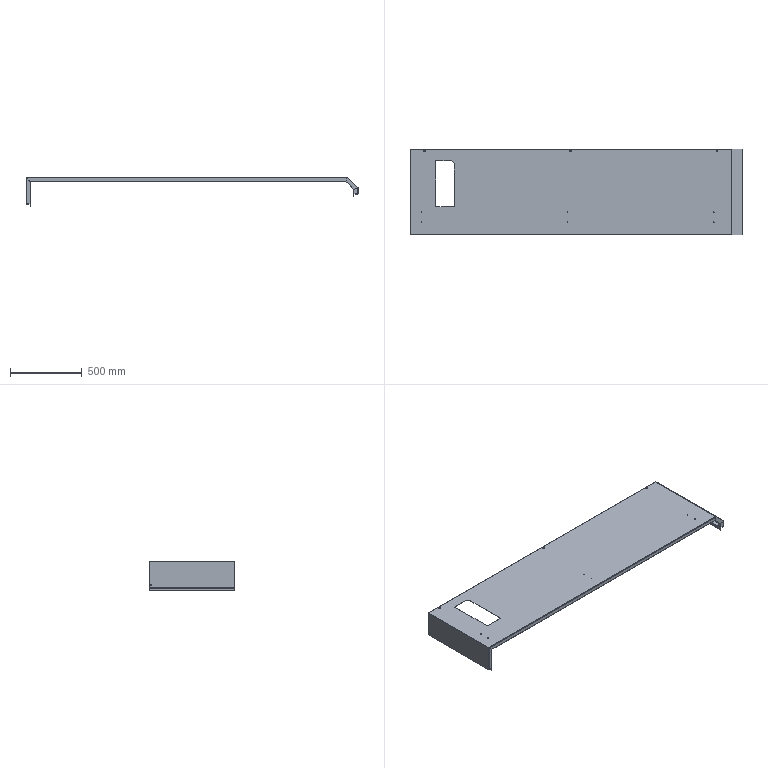Part | STEP file | Front Panel | 1 solid | 237 faces | box 2314 x 597 x 206.5 mm | volume 2666967 mm3 | plane 128 | cylinder 97 | spline 12 | commonest cylinder face diameters 1 x23 4 x23 0.15 x18 6 x12 7 x10 13 x10